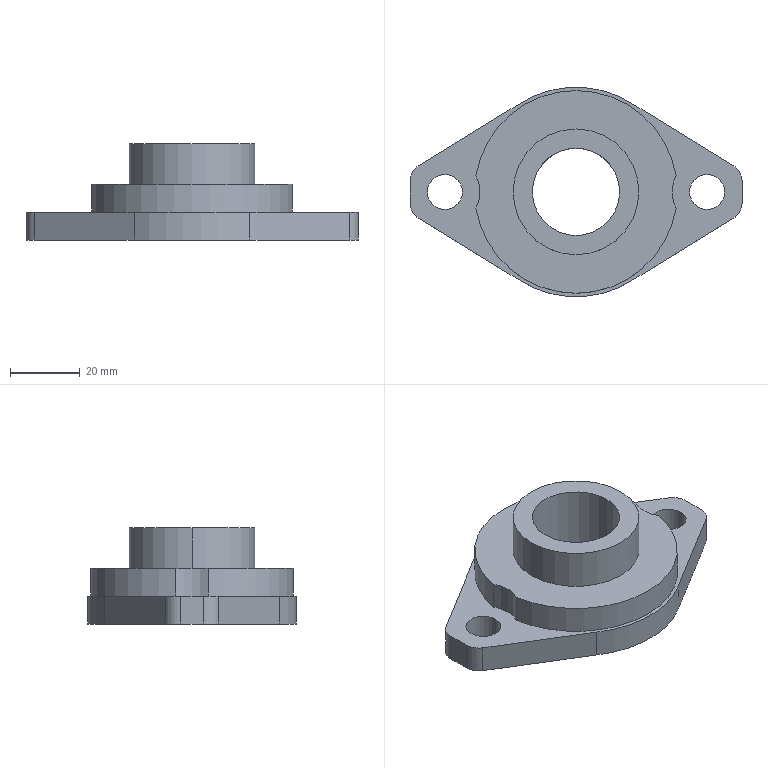Part | SolidWorks | features BaseBody 1 | 1 solid | 32 faces | box 95 x 60 x 27.5 mm | volume 44530 mm3 | cylinder 21 | plane 11 | commonest cylinder face diameters 10 x8 20 x3 25 x2 36 x2 55 x2 58 x2
STEP:
#1=CARTESIAN_POINT('',(12.5,0.,19.5));
#2=VERTEX_POINT('',#1);
#3=CARTESIAN_POINT('',(-12.5,0.,19.5));
#4=VERTEX_POINT('',#3);
#5=CARTESIAN_POINT('',(0.,0.,19.5));
#6=DIRECTION('',(0.,0.,-1.));
#7=DIRECTION('',(-1.,0.,0.));
#8=AXIS2_PLACEMENT_3D('',#5,#6,#7);
#9=CIRCLE('',#8,12.5);
#10=EDGE_CURVE('',#2,#4,#9,.T.);
#11=ORIENTED_EDGE('',*,*,#10,.F.);
#12=CARTESIAN_POINT('',(12.5,0.,-6.));
#13=VERTEX_POINT('',#12);
#14=CARTESIAN_POINT('',(12.5,0.,19.5));
#15=DIRECTION('',(0.,0.,-1.));
#16=VECTOR('',#15,1000.);
#17=LINE('',#14,#16);
#18=EDGE_CURVE('',#2,#13,#17,.T.);
#19=ORIENTED_EDGE('',*,*,#18,.T.);
#20=CARTESIAN_POINT('',(-12.5,0.,-6.));
#21=VERTEX_POINT('',#20);
#22=CARTESIAN_POINT('',(0.,0.,-6.));
#23=DIRECTION('',(0.,0.,1.));
#24=DIRECTION('',(-1.,0.,0.));
#25=AXIS2_PLACEMENT_3D('',#22,#23,#24);
#26=CIRCLE('',#25,12.5);
#27=EDGE_CURVE('',#21,#13,#26,.T.);
#28=ORIENTED_EDGE('',*,*,#27,.F.);
#29=CARTESIAN_POINT('',(-12.5,0.,19.5));
#30=DIRECTION('',(0.,0.,-1.));
#31=VECTOR('',#30,1000.);
#32=LINE('',#29,#31);
#33=EDGE_CURVE('',#4,#21,#32,.T.);
#34=ORIENTED_EDGE('',*,*,#33,.F.);
#35=EDGE_LOOP('',(#11,#19,#28,#34));
#36=FACE_OUTER_BOUND('',#35,.T.);
#37=CARTESIAN_POINT('',(0.,0.,19.5));
#38=DIRECTION('',(0.,0.,-1.));
#39=DIRECTION('',(-1.,0.,0.));
#40=AXIS2_PLACEMENT_3D('',#37,#38,#39);
#41=CYLINDRICAL_SURFACE('',#40,12.5);
#42=ADVANCED_FACE('',(#36),#41,.F.);
#43=CARTESIAN_POINT('',(18.,0.,8.));
#44=VERTEX_POINT('',#43);
#45=CARTESIAN_POINT('',(-18.,0.,8.));
#46=VERTEX_POINT('',#45);
#47=CARTESIAN_POINT('',(0.,0.,8.));
#48=DIRECTION('',(0.,0.,1.));
#49=DIRECTION('',(1.,0.,0.));
#50=AXIS2_PLACEMENT_3D('',#47,#48,#49);
#51=CIRCLE('',#50,18.);
#52=EDGE_CURVE('',#44,#46,#51,.T.);
#53=ORIENTED_EDGE('',*,*,#52,.T.);
#54=CARTESIAN_POINT('',(-18.,0.,19.5));
#55=VERTEX_POINT('',#54);
#56=CARTESIAN_POINT('',(-18.,0.,8.));
#57=DIRECTION('',(0.,0.,1.));
#58=VECTOR('',#57,1000.);
#59=LINE('',#56,#58);
#60=EDGE_CURVE('',#46,#55,#59,.T.);
#61=ORIENTED_EDGE('',*,*,#60,.T.);
#62=CARTESIAN_POINT('',(18.,0.,19.5));
#63=VERTEX_POINT('',#62);
#64=CARTESIAN_POINT('',(0.,0.,19.5));
#65=DIRECTION('',(0.,0.,1.));
#66=DIRECTION('',(1.,0.,0.));
#67=AXIS2_PLACEMENT_3D('',#64,#65,#66);
#68=CIRCLE('',#67,18.);
#69=EDGE_CURVE('',#63,#55,#68,.T.);
#70=ORIENTED_EDGE('',*,*,#69,.F.);
#71=CARTESIAN_POINT('',(18.,0.,8.));
#72=DIRECTION('',(0.,0.,1.));
#73=VECTOR('',#72,1000.);
#74=LINE('',#71,#73);
#75=EDGE_CURVE('',#44,#63,#74,.T.);
#76=ORIENTED_EDGE('',*,*,#75,.F.);
#77=EDGE_LOOP('',(#53,#61,#70,#76));
#78=FACE_OUTER_BOUND('',#77,.T.);
#79=CARTESIAN_POINT('',(0.,0.,8.));
#80=DIRECTION('',(0.,0.,1.));
#81=DIRECTION('',(1.,0.,0.));
#82=AXIS2_PLACEMENT_3D('',#79,#80,#81);
#83=CYLINDRICAL_SURFACE('',#82,18.);
#84=ADVANCED_FACE('',(#78),#83,.T.);
#85=CARTESIAN_POINT('',(-27.5,0.,-8.));
#86=VERTEX_POINT('',#85);
#87=CARTESIAN_POINT('',(27.5,0.,-8.));
#88=VERTEX_POINT('',#87);
#89=CARTESIAN_POINT('',(0.,0.,-8.));
#90=DIRECTION('',(0.,0.,1.));
#91=DIRECTION('',(1.,0.,0.));
#92=AXIS2_PLACEMENT_3D('',#89,#90,#91);
#93=CIRCLE('',#92,27.5);
#94=EDGE_CURVE('',#86,#88,#93,.T.);
#95=ORIENTED_EDGE('',*,*,#94,.F.);
#96=CARTESIAN_POINT('',(-27.5,0.,-6.));
#97=VERTEX_POINT('',#96);
#98=CARTESIAN_POINT('',(-27.5,0.,-8.));
#99=DIRECTION('',(0.,0.,1.));
#100=VECTOR('',#99,1000.);
#101=LINE('',#98,#100);
#102=EDGE_CURVE('',#86,#97,#101,.T.);
#103=ORIENTED_EDGE('',*,*,#102,.T.);
#104=CARTESIAN_POINT('',(27.5,0.,-6.));
#105=VERTEX_POINT('',#104);
#106=CARTESIAN_POINT('',(0.,0.,-6.));
#107=DIRECTION('',(0.,0.,1.));
#108=DIRECTION('',(1.,0.,0.));
#109=AXIS2_PLACEMENT_3D('',#106,#107,#108);
#110=CIRCLE('',#109,27.5);
#111=EDGE_CURVE('',#97,#105,#110,.T.);
#112=ORIENTED_EDGE('',*,*,#111,.T.);
#113=CARTESIAN_POINT('',(27.5,0.,-8.));
#114=DIRECTION('',(0.,0.,1.));
#115=VECTOR('',#114,1000.);
#116=LINE('',#113,#115);
#117=EDGE_CURVE('',#88,#105,#116,.T.);
#118=ORIENTED_EDGE('',*,*,#117,.F.);
#119=EDGE_LOOP('',(#95,#103,#112,#118));
#120=FACE_OUTER_BOUND('',#119,.T.);
#121=CARTESIAN_POINT('',(0.,0.,-8.));
#122=DIRECTION('',(0.,0.,1.));
#123=DIRECTION('',(1.,0.,0.));
#124=AXIS2_PLACEMENT_3D('',#121,#122,#123);
#125=CYLINDRICAL_SURFACE('',#124,27.5);
#126=ADVANCED_FACE('',(#120),#125,.F.);
#127=CARTESIAN_POINT('',(27.5,0.,8.));
#128=VERTEX_POINT('',#127);
#129=CARTESIAN_POINT('',(28.63,4.618,8.));
#130=VERTEX_POINT('',#129);
#131=CARTESIAN_POINT('',(37.5,0.,8.));
#132=DIRECTION('',(0.,0.,-1.));
#133=DIRECTION('',(-1.,0.,0.));
#134=AXIS2_PLACEMENT_3D('',#131,#132,#133);
#135=CIRCLE('',#134,10.);
#136=EDGE_CURVE('',#128,#130,#135,.T.);
#137=ORIENTED_EDGE('',*,*,#136,.F.);
#138=CARTESIAN_POINT('',(27.5,0.,0.));
#139=VERTEX_POINT('',#138);
#140=CARTESIAN_POINT('',(27.5,0.,8.));
#141=DIRECTION('',(0.,0.,-1.));
#142=VECTOR('',#141,1000.);
#143=LINE('',#140,#142);
#144=EDGE_CURVE('',#128,#139,#143,.T.);
#145=ORIENTED_EDGE('',*,*,#144,.T.);
#146=CARTESIAN_POINT('',(28.63,4.618,0.));
#147=VERTEX_POINT('',#146);
#148=CARTESIAN_POINT('',(37.5,0.,0.));
#149=DIRECTION('',(0.,0.,1.));
#150=DIRECTION('',(-1.,0.,0.));
#151=AXIS2_PLACEMENT_3D('',#148,#149,#150);
#152=CIRCLE('',#151,10.);
#153=EDGE_CURVE('',#147,#139,#152,.T.);
#154=ORIENTED_EDGE('',*,*,#153,.F.);
#155=CARTESIAN_POINT('',(28.63,4.618,0.));
#156=DIRECTION('',(0.,0.,-1.));
#157=VECTOR('',#156,1000.);
#158=LINE('',#155,#157);
#159=EDGE_CURVE('',#130,#147,#158,.T.);
#160=ORIENTED_EDGE('',*,*,#159,.F.);
#161=EDGE_LOOP('',(#137,#145,#154,#160));
#162=FACE_OUTER_BOUND('',#161,.T.);
#163=CARTESIAN_POINT('',(37.5,0.,8.));
#164=DIRECTION('',(0.,0.,-1.));
#165=DIRECTION('',(-1.,0.,0.));
#166=AXIS2_PLACEMENT_3D('',#163,#164,#165);
#167=CYLINDRICAL_SURFACE('',#166,10.);
#168=ADVANCED_FACE('',(#162),#167,.F.);
#169=CARTESIAN_POINT('',(32.5,0.,-8.));
#170=VERTEX_POINT('',#169);
#171=CARTESIAN_POINT('',(42.5,0.,-8.));
#172=VERTEX_POINT('',#171);
#173=CARTESIAN_POINT('',(37.5,0.,-8.));
#174=DIRECTION('',(0.,0.,1.));
#175=DIRECTION('',(1.,0.,0.));
#176=AXIS2_PLACEMENT_3D('',#173,#174,#175);
#177=CIRCLE('',#176,5.);
#178=EDGE_CURVE('',#170,#172,#177,.T.);
#179=ORIENTED_EDGE('',*,*,#178,.F.);
#180=CARTESIAN_POINT('',(32.5,0.,0.));
#181=VERTEX_POINT('',#180);
#182=CARTESIAN_POINT('',(32.5,0.,-8.));
#183=DIRECTION('',(0.,0.,1.));
#184=VECTOR('',#183,1000.);
#185=LINE('',#182,#184);
#186=EDGE_CURVE('',#170,#181,#185,.T.);
#187=ORIENTED_EDGE('',*,*,#186,.T.);
#188=CARTESIAN_POINT('',(42.5,0.,0.));
#189=VERTEX_POINT('',#188);
#190=CARTESIAN_POINT('',(37.5,0.,0.));
#191=DIRECTION('',(0.,0.,-1.));
#192=DIRECTION('',(1.,0.,0.));
#193=AXIS2_PLACEMENT_3D('',#190,#191,#192);
#194=CIRCLE('',#193,5.);
#195=EDGE_CURVE('',#189,#181,#194,.T.);
#196=ORIENTED_EDGE('',*,*,#195,.F.);
#197=CARTESIAN_POINT('',(42.5,0.,-8.));
#198=DIRECTION('',(0.,0.,1.));
#199=VECTOR('',#198,1000.);
#200=LINE('',#197,#199);
#201=EDGE_CURVE('',#172,#189,#200,.T.);
#202=ORIENTED_EDGE('',*,*,#201,.F.);
#203=EDGE_LOOP('',(#179,#187,#196,#202));
#204=FACE_OUTER_BOUND('',#203,.T.);
#205=CARTESIAN_POINT('',(37.5,0.,-8.));
#206=DIRECTION('',(0.,0.,1.));
#207=DIRECTION('',(1.,0.,0.));
#208=AXIS2_PLACEMENT_3D('',#205,#206,#207);
#209=CYLINDRICAL_SURFACE('',#208,5.);
#210=ADVANCED_FACE('',(#204),#209,.F.);
#211=CARTESIAN_POINT('',(-42.5,0.,-8.));
#212=VERTEX_POINT('',#211);
#213=CARTESIAN_POINT('',(-32.5,0.,-8.));
#214=VERTEX_POINT('',#213);
#215=CARTESIAN_POINT('',(-37.5,0.,-8.));
#216=DIRECTION('',(0.,0.,1.));
#217=DIRECTION('',(1.,0.,0.));
#218=AXIS2_PLACEMENT_3D('',#215,#216,#217);
#219=CIRCLE('',#218,5.);
#220=EDGE_CURVE('',#212,#214,#219,.T.);
#221=ORIENTED_EDGE('',*,*,#220,.F.);
#222=CARTESIAN_POINT('',(-42.5,0.,0.));
#223=VERTEX_POINT('',#222);
#224=CARTESIAN_POINT('',(-42.5,0.,-8.));
#225=DIRECTION('',(0.,0.,1.));
#226=VECTOR('',#225,1000.);
#227=LINE('',#224,#226);
#228=EDGE_CURVE('',#212,#223,#227,.T.);
#229=ORIENTED_EDGE('',*,*,#228,.T.);
#230=CARTESIAN_POINT('',(-32.5,0.,0.));
#231=VERTEX_POINT('',#230);
#232=CARTESIAN_POINT('',(-37.5,0.,0.));
#233=DIRECTION('',(0.,0.,-1.));
#234=DIRECTION('',(1.,0.,0.));
#235=AXIS2_PLACEMENT_3D('',#232,#233,#234);
#236=CIRCLE('',#235,5.);
#237=EDGE_CURVE('',#231,#223,#236,.T.);
#238=ORIENTED_EDGE('',*,*,#237,.F.);
#239=CARTESIAN_POINT('',(-32.5,0.,-8.));
#240=DIRECTION('',(0.,0.,1.));
#241=VECTOR('',#240,1000.);
#242=LINE('',#239,#241);
#243=EDGE_CURVE('',#214,#231,#242,.T.);
#244=ORIENTED_EDGE('',*,*,#243,.F.);
#245=EDGE_LOOP('',(#221,#229,#238,#244));
#246=FACE_OUTER_BOUND('',#245,.T.);
#247=CARTESIAN_POINT('',(-37.5,0.,-8.));
#248=DIRECTION('',(0.,0.,1.));
#249=DIRECTION('',(1.,0.,0.));
#250=AXIS2_PLACEMENT_3D('',#247,#248,#249);
#251=CYLINDRICAL_SURFACE('',#250,5.);
#252=ADVANCED_FACE('',(#246),#251,.F.);
#253=ORIENTED_EDGE('',*,*,#18,.F.);
#254=CARTESIAN_POINT('',(0.,0.,19.5));
#255=DIRECTION('',(0.,0.,-1.));
#256=DIRECTION('',(-1.,0.,0.));
#257=AXIS2_PLACEMENT_3D('',#254,#255,#256);
#258=CIRCLE('',#257,12.5);
#259=EDGE_CURVE('',#4,#2,#258,.T.);
#260=ORIENTED_EDGE('',*,*,#259,.F.);
#261=ORIENTED_EDGE('',*,*,#33,.T.);
#262=CARTESIAN_POINT('',(0.,0.,-6.));
#263=DIRECTION('',(0.,0.,1.));
#264=DIRECTION('',(-1.,0.,0.));
#265=AXIS2_PLACEMENT_3D('',#262,#263,#264);
#266=CIRCLE('',#265,12.5);
#267=EDGE_CURVE('',#13,#21,#266,.T.);
#268=ORIENTED_EDGE('',*,*,#267,.F.);
#269=EDGE_LOOP('',(#253,#260,#261,#268));
#270=FACE_OUTER_BOUND('',#269,.T.);
#271=CARTESIAN_POINT('',(0.,0.,19.5));
#272=DIRECTION('',(0.,0.,-1.));
#273=DIRECTION('',(-1.,0.,0.));
#274=AXIS2_PLACEMENT_3D('',#271,#272,#273);
#275=CYLINDRICAL_SURFACE('',#274,12.5);
#276=ADVANCED_FACE('',(#270),#275,.F.);
#277=ORIENTED_EDGE('',*,*,#69,.T.);
#278=CARTESIAN_POINT('',(0.,0.,19.5));
#279=DIRECTION('',(0.,0.,1.));
#280=DIRECTION('',(1.,0.,0.));
#281=AXIS2_PLACEMENT_3D('',#278,#279,#280);
#282=CIRCLE('',#281,18.);
#283=EDGE_CURVE('',#55,#63,#282,.T.);
#284=ORIENTED_EDGE('',*,*,#283,.T.);
#285=EDGE_LOOP('',(#277,#284));
#286=FACE_OUTER_BOUND('',#285,.T.);
#287=ORIENTED_EDGE('',*,*,#259,.T.);
#288=ORIENTED_EDGE('',*,*,#10,.T.);
#289=EDGE_LOOP('',(#287,#288));
#290=FACE_BOUND('',#289,.T.);
#291=CARTESIAN_POINT('',(0.,0.,19.5));
#292=DIRECTION('',(0.,0.,1.));
#293=DIRECTION('',(1.,0.,0.));
#294=AXIS2_PLACEMENT_3D('',#291,#292,#293);
#295=PLANE('',#294);
#296=ADVANCED_FACE('',(#286,#290),#295,.T.);
#297=ORIENTED_EDGE('',*,*,#27,.T.);
#298=ORIENTED_EDGE('',*,*,#267,.T.);
#299=EDGE_LOOP('',(#297,#298));
#300=FACE_BOUND('',#299,.T.);
#301=CARTESIAN_POINT('',(0.,0.,-6.));
#302=DIRECTION('',(0.,0.,1.));
#303=DIRECTION('',(1.,0.,0.));
#304=AXIS2_PLACEMENT_3D('',#301,#302,#303);
#305=CIRCLE('',#304,27.5);
#306=EDGE_CURVE('',#105,#97,#305,.T.);
#307=ORIENTED_EDGE('',*,*,#306,.F.);
#308=ORIENTED_EDGE('',*,*,#111,.F.);
#309=EDGE_LOOP('',(#307,#308));
#310=FACE_OUTER_BOUND('',#309,.T.);
#311=CARTESIAN_POINT('',(0.,0.,-6.));
#312=DIRECTION('',(0.,0.,1.));
#313=DIRECTION('',(1.,0.,0.));
#314=AXIS2_PLACEMENT_3D('',#311,#312,#313);
#315=PLANE('',#314);
#316=ADVANCED_FACE('',(#300,#310),#315,.F.);
#317=ORIENTED_EDGE('',*,*,#60,.F.);
#318=CARTESIAN_POINT('',(0.,0.,8.));
#319=DIRECTION('',(0.,0.,1.));
#320=DIRECTION('',(1.,0.,0.));
#321=AXIS2_PLACEMENT_3D('',#318,#319,#320);
#322=CIRCLE('',#321,18.);
#323=EDGE_CURVE('',#46,#44,#322,.T.);
#324=ORIENTED_EDGE('',*,*,#323,.T.);
#325=ORIENTED_EDGE('',*,*,#75,.T.);
#326=ORIENTED_EDGE('',*,*,#283,.F.);
#327=EDGE_LOOP('',(#317,#324,#325,#326));
#328=FACE_OUTER_BOUND('',#327,.T.);
#329=CARTESIAN_POINT('',(0.,0.,8.));
#330=DIRECTION('',(0.,0.,1.));
#331=DIRECTION('',(1.,0.,0.));
#332=AXIS2_PLACEMENT_3D('',#329,#330,#331);
#333=CYLINDRICAL_SURFACE('',#332,18.);
#334=ADVANCED_FACE('',(#328),#333,.T.);
#335=ORIENTED_EDGE('',*,*,#102,.F.);
#336=CARTESIAN_POINT('',(0.,0.,-8.));
#337=DIRECTION('',(0.,0.,1.));
#338=DIRECTION('',(1.,0.,0.));
#339=AXIS2_PLACEMENT_3D('',#336,#337,#338);
#340=CIRCLE('',#339,27.5);
#341=EDGE_CURVE('',#88,#86,#340,.T.);
#342=ORIENTED_EDGE('',*,*,#341,.F.);
#343=ORIENTED_EDGE('',*,*,#117,.T.);
#344=ORIENTED_EDGE('',*,*,#306,.T.);
#345=EDGE_LOOP('',(#335,#342,#343,#344));
#346=FACE_OUTER_BOUND('',#345,.T.);
#347=CARTESIAN_POINT('',(0.,0.,-8.));
#348=DIRECTION('',(0.,0.,1.));
#349=DIRECTION('',(1.,0.,0.));
#350=AXIS2_PLACEMENT_3D('',#347,#348,#349);
#351=CYLINDRICAL_SURFACE('',#350,27.5);
#352=ADVANCED_FACE('',(#346),#351,.F.);
#353=ORIENTED_EDGE('',*,*,#52,.F.);
#354=ORIENTED_EDGE('',*,*,#323,.F.);
#355=EDGE_LOOP('',(#353,#354));
#356=FACE_BOUND('',#355,.T.);
#357=CARTESIAN_POINT('',(-28.63,4.618,8.));
#358=VERTEX_POINT('',#357);
#359=CARTESIAN_POINT('',(-28.63,-4.618,8.));
#360=VERTEX_POINT('',#359);
#361=CARTESIAN_POINT('',(-37.5,0.,8.));
#362=DIRECTION('',(0.,0.,-1.));
#363=DIRECTION('',(-1.,0.,0.));
#364=AXIS2_PLACEMENT_3D('',#361,#362,#363);
#365=CIRCLE('',#364,10.);
#366=EDGE_CURVE('',#358,#360,#365,.T.);
#367=ORIENTED_EDGE('',*,*,#366,.T.);
#368=CARTESIAN_POINT('',(28.63,-4.618,8.));
#369=VERTEX_POINT('',#368);
#370=CARTESIAN_POINT('',(0.,0.,8.));
#371=DIRECTION('',(0.,0.,1.));
#372=DIRECTION('',(1.,0.,0.));
#373=AXIS2_PLACEMENT_3D('',#370,#371,#372);
#374=CIRCLE('',#373,29.);
#375=EDGE_CURVE('',#360,#369,#374,.T.);
#376=ORIENTED_EDGE('',*,*,#375,.T.);
#377=CARTESIAN_POINT('',(37.5,0.,8.));
#378=DIRECTION('',(0.,0.,-1.));
#379=DIRECTION('',(-1.,0.,0.));
#380=AXIS2_PLACEMENT_3D('',#377,#378,#379);
#381=CIRCLE('',#380,10.);
#382=EDGE_CURVE('',#369,#128,#381,.T.);
#383=ORIENTED_EDGE('',*,*,#382,.T.);
#384=ORIENTED_EDGE('',*,*,#136,.T.);
#385=CARTESIAN_POINT('',(0.,0.,8.));
#386=DIRECTION('',(0.,0.,1.));
#387=DIRECTION('',(1.,0.,0.));
#388=AXIS2_PLACEMENT_3D('',#385,#386,#387);
#389=CIRCLE('',#388,29.);
#390=EDGE_CURVE('',#130,#358,#389,.T.);
#391=ORIENTED_EDGE('',*,*,#390,.T.);
#392=EDGE_LOOP('',(#367,#376,#383,#384,#391));
#393=FACE_OUTER_BOUND('',#392,.T.);
#394=CARTESIAN_POINT('',(0.,0.,8.));
#395=DIRECTION('',(0.,0.,1.));
#396=DIRECTION('',(1.,0.,0.));
#397=AXIS2_PLACEMENT_3D('',#394,#395,#396);
#398=PLANE('',#397);
#399=ADVANCED_FACE('',(#356,#393),#398,.T.);
#400=CARTESIAN_POINT('',(37.5,0.,-8.));
#401=DIRECTION('',(0.,0.,1.));
#402=DIRECTION('',(1.,0.,0.));
#403=AXIS2_PLACEMENT_3D('',#400,#401,#402);
#404=CIRCLE('',#403,5.);
#405=EDGE_CURVE('',#172,#170,#404,.T.);
#406=ORIENTED_EDGE('',*,*,#405,.T.);
#407=ORIENTED_EDGE('',*,*,#178,.T.);
#408=EDGE_LOOP('',(#406,#407));
#409=FACE_BOUND('',#408,.T.);
#410=CARTESIAN_POINT('',(-37.5,0.,-8.));
#411=DIRECTION('',(0.,0.,1.));
#412=DIRECTION('',(1.,0.,0.));
#413=AXIS2_PLACEMENT_3D('',#410,#411,#412);
#414=CIRCLE('',#413,5.);
#415=EDGE_CURVE('',#214,#212,#414,.T.);
#416=ORIENTED_EDGE('',*,*,#415,.T.);
#417=ORIENTED_EDGE('',*,*,#220,.T.);
#418=EDGE_LOOP('',(#416,#417));
#419=FACE_BOUND('',#418,.T.);
#420=CARTESIAN_POINT('',(16.583,25.,-8.));
#421=VERTEX_POINT('',#420);
#422=CARTESIAN_POINT('',(45.118,7.464,-8.));
#423=VERTEX_POINT('',#422);
#424=CARTESIAN_POINT('',(16.583,25.,-8.));
#425=DIRECTION('',(0.852,-0.5236,0.));
#426=VECTOR('',#425,1000.);
#427=LINE('',#424,#426);
#428=EDGE_CURVE('',#421,#423,#427,.T.);
#429=ORIENTED_EDGE('',*,*,#428,.T.);
#430=CARTESIAN_POINT('',(47.5,3.204,-8.));
#431=VERTEX_POINT('',#430);
#432=CARTESIAN_POINT('',(42.5,3.204,-8.));
#433=DIRECTION('',(0.,0.,-1.));
#434=DIRECTION('',(1.,0.,0.));
#435=AXIS2_PLACEMENT_3D('',#432,#433,#434);
#436=CIRCLE('',#435,5.);
#437=EDGE_CURVE('',#423,#431,#436,.T.);
#438=ORIENTED_EDGE('',*,*,#437,.T.);
#439=CARTESIAN_POINT('',(47.5,-3.204,-8.));
#440=VERTEX_POINT('',#439);
#441=CARTESIAN_POINT('',(47.5,0.,-8.));
#442=DIRECTION('',(0.,-1.,0.));
#443=VECTOR('',#442,1000.);
#444=LINE('',#441,#443);
#445=EDGE_CURVE('',#431,#440,#444,.T.);
#446=ORIENTED_EDGE('',*,*,#445,.T.);
#447=CARTESIAN_POINT('',(45.118,-7.464,-8.));
#448=VERTEX_POINT('',#447);
#449=CARTESIAN_POINT('',(42.5,-3.204,-8.));
#450=DIRECTION('',(0.,0.,-1.));
#451=DIRECTION('',(1.,0.,0.));
#452=AXIS2_PLACEMENT_3D('',#449,#450,#451);
#453=CIRCLE('',#452,5.);
#454=EDGE_CURVE('',#440,#448,#453,.T.);
#455=ORIENTED_EDGE('',*,*,#454,.T.);
#456=CARTESIAN_POINT('',(16.583,-25.,-8.));
#457=VERTEX_POINT('',#456);
#458=CARTESIAN_POINT('',(45.118,-7.464,-8.));
#459=DIRECTION('',(-0.852,-0.5236,0.));
#460=VECTOR('',#459,1000.);
#461=LINE('',#458,#460);
#462=EDGE_CURVE('',#448,#457,#461,.T.);
#463=ORIENTED_EDGE('',*,*,#462,.T.);
#464=CARTESIAN_POINT('',(-16.583,-25.,-8.));
#465=VERTEX_POINT('',#464);
#466=CARTESIAN_POINT('',(0.,0.,-8.));
#467=DIRECTION('',(0.,0.,-1.));
#468=DIRECTION('',(1.,0.,0.));
#469=AXIS2_PLACEMENT_3D('',#466,#467,#468);
#470=CIRCLE('',#469,30.);
#471=EDGE_CURVE('',#457,#465,#470,.T.);
#472=ORIENTED_EDGE('',*,*,#471,.T.);
#473=CARTESIAN_POINT('',(-45.118,-7.464,-8.));
#474=VERTEX_POINT('',#473);
#475=CARTESIAN_POINT('',(-16.583,-25.,-8.));
#476=DIRECTION('',(-0.852,0.5236,0.));
#477=VECTOR('',#476,1000.);
#478=LINE('',#475,#477);
#479=EDGE_CURVE('',#465,#474,#478,.T.);
#480=ORIENTED_EDGE('',*,*,#479,.T.);
#481=CARTESIAN_POINT('',(-47.5,-3.204,-8.));
#482=VERTEX_POINT('',#481);
#483=CARTESIAN_POINT('',(-42.5,-3.204,-8.));
#484=DIRECTION('',(0.,0.,-1.));
#485=DIRECTION('',(1.,0.,0.));
#486=AXIS2_PLACEMENT_3D('',#483,#484,#485);
#487=CIRCLE('',#486,5.);
#488=EDGE_CURVE('',#474,#482,#487,.T.);
#489=ORIENTED_EDGE('',*,*,#488,.T.);
#490=CARTESIAN_POINT('',(-47.5,3.204,-8.));
#491=VERTEX_POINT('',#490);
#492=CARTESIAN_POINT('',(-47.5,0.,-8.));
#493=DIRECTION('',(0.,1.,0.));
#494=VECTOR('',#493,1000.);
#495=LINE('',#492,#494);
#496=EDGE_CURVE('',#482,#491,#495,.T.);
#497=ORIENTED_EDGE('',*,*,#496,.T.);
#498=CARTESIAN_POINT('',(-45.118,7.464,-8.));
#499=VERTEX_POINT('',#498);
#500=CARTESIAN_POINT('',(-42.5,3.204,-8.));
#501=DIRECTION('',(0.,0.,-1.));
#502=DIRECTION('',(1.,0.,0.));
#503=AXIS2_PLACEMENT_3D('',#500,#501,#502);
#504=CIRCLE('',#503,5.);
#505=EDGE_CURVE('',#491,#499,#504,.T.);
#506=ORIENTED_EDGE('',*,*,#505,.T.);
#507=CARTESIAN_POINT('',(-16.583,25.,-8.));
#508=VERTEX_POINT('',#507);
#509=CARTESIAN_POINT('',(-45.118,7.464,-8.));
#510=DIRECTION('',(0.852,0.5236,0.));
#511=VECTOR('',#510,1000.);
#512=LINE('',#509,#511);
#513=EDGE_CURVE('',#499,#508,#512,.T.);
#514=ORIENTED_EDGE('',*,*,#513,.T.);
#515=CARTESIAN_POINT('',(0.,0.,-8.));
#516=DIRECTION('',(0.,0.,-1.));
#517=DIRECTION('',(1.,0.,0.));
#518=AXIS2_PLACEMENT_3D('',#515,#516,#517);
#519=CIRCLE('',#518,30.);
#520=EDGE_CURVE('',#508,#421,#519,.T.);
#521=ORIENTED_EDGE('',*,*,#520,.T.);
#522=EDGE_LOOP('',(#429,#438,#446,#455,#463,#472,#480,#489,#497,#506,#514,#521));
#523=FACE_OUTER_BOUND('',#522,.T.);
#524=ORIENTED_EDGE('',*,*,#341,.T.);
#525=ORIENTED_EDGE('',*,*,#94,.T.);
#526=EDGE_LOOP('',(#524,#525));
#527=FACE_BOUND('',#526,.T.);
#528=CARTESIAN_POINT('',(0.,0.,-8.));
#529=DIRECTION('',(0.,0.,-1.));
#530=DIRECTION('',(-1.,0.,0.));
#531=AXIS2_PLACEMENT_3D('',#528,#529,#530);
#532=PLANE('',#531);
#533=ADVANCED_FACE('',(#409,#419,#523,#527),#532,.T.);
#534=CARTESIAN_POINT('',(-28.63,-4.618,0.));
#535=VERTEX_POINT('',#534);
#536=CARTESIAN_POINT('',(-28.63,-4.618,0.));
#537=DIRECTION('',(0.,0.,-1.));
#538=VECTOR('',#537,1000.);
#539=LINE('',#536,#538);
#540=EDGE_CURVE('',#360,#535,#539,.T.);
#541=ORIENTED_EDGE('',*,*,#540,.T.);
#542=CARTESIAN_POINT('',(28.63,-4.618,0.));
#543=VERTEX_POINT('',#542);
#544=CARTESIAN_POINT('',(0.,0.,0.));
#545=DIRECTION('',(0.,0.,1.));
#546=DIRECTION('',(1.,0.,0.));
#547=AXIS2_PLACEMENT_3D('',#544,#545,#546);
#548=CIRCLE('',#547,29.);
#549=EDGE_CURVE('',#535,#543,#548,.T.);
#550=ORIENTED_EDGE('',*,*,#549,.T.);
#551=CARTESIAN_POINT('',(28.63,-4.618,0.));
#552=DIRECTION('',(0.,0.,1.));
#553=VECTOR('',#552,1000.);
#554=LINE('',#551,#553);
#555=EDGE_CURVE('',#543,#369,#554,.T.);
#556=ORIENTED_EDGE('',*,*,#555,.T.);
#557=ORIENTED_EDGE('',*,*,#375,.F.);
#558=EDGE_LOOP('',(#541,#550,#556,#557));
#559=FACE_OUTER_BOUND('',#558,.T.);
#560=CARTESIAN_POINT('',(0.,0.,0.));
#561=DIRECTION('',(0.,0.,1.));
#562=DIRECTION('',(1.,0.,0.));
#563=AXIS2_PLACEMENT_3D('',#560,#561,#562);
#564=CYLINDRICAL_SURFACE('',#563,29.);
#565=ADVANCED_FACE('',(#559),#564,.T.);
#566=ORIENTED_EDGE('',*,*,#366,.F.);
#567=CARTESIAN_POINT('',(-28.63,4.618,0.));
#568=VERTEX_POINT('',#567);
#569=CARTESIAN_POINT('',(-28.63,4.618,8.));
#570=DIRECTION('',(0.,0.,1.));
#571=VECTOR('',#570,1000.);
#572=LINE('',#569,#571);
#573=EDGE_CURVE('',#568,#358,#572,.T.);
#574=ORIENTED_EDGE('',*,*,#573,.F.);
#575=CARTESIAN_POINT('',(-37.5,0.,0.));
#576=DIRECTION('',(0.,0.,1.));
#577=DIRECTION('',(-1.,0.,0.));
#578=AXIS2_PLACEMENT_3D('',#575,#576,#577);
#579=CIRCLE('',#578,10.);
#580=EDGE_CURVE('',#535,#568,#579,.T.);
#581=ORIENTED_EDGE('',*,*,#580,.F.);
#582=ORIENTED_EDGE('',*,*,#540,.F.);
#583=EDGE_LOOP('',(#566,#574,#581,#582));
#584=FACE_OUTER_BOUND('',#583,.T.);
#585=CARTESIAN_POINT('',(-37.5,0.,8.));
#586=DIRECTION('',(0.,0.,-1.));
#587=DIRECTION('',(-1.,0.,0.));
#588=AXIS2_PLACEMENT_3D('',#585,#586,#587);
#589=CYLINDRICAL_SURFACE('',#588,10.);
#590=ADVANCED_FACE('',(#584),#589,.F.);
#591=ORIENTED_EDGE('',*,*,#573,.T.);
#592=ORIENTED_EDGE('',*,*,#390,.F.);
#593=ORIENTED_EDGE('',*,*,#159,.T.);
#594=CARTESIAN_POINT('',(0.,0.,0.));
#595=DIRECTION('',(0.,0.,1.));
#596=DIRECTION('',(1.,0.,0.));
#597=AXIS2_PLACEMENT_3D('',#594,#595,#596);
#598=CIRCLE('',#597,29.);
#599=EDGE_CURVE('',#147,#568,#598,.T.);
#600=ORIENTED_EDGE('',*,*,#599,.T.);
#601=EDGE_LOOP('',(#591,#592,#593,#600));
#602=FACE_OUTER_BOUND('',#601,.T.);
#603=CARTESIAN_POINT('',(0.,0.,0.));
#604=DIRECTION('',(0.,0.,1.));
#605=DIRECTION('',(1.,0.,0.));
#606=AXIS2_PLACEMENT_3D('',#603,#604,#605);
#607=CYLINDRICAL_SURFACE('',#606,29.);
#608=ADVANCED_FACE('',(#602),#607,.T.);
#609=ORIENTED_EDGE('',*,*,#144,.F.);
#610=ORIENTED_EDGE('',*,*,#382,.F.);
#611=ORIENTED_EDGE('',*,*,#555,.F.);
#612=CARTESIAN_POINT('',(37.5,0.,0.));
#613=DIRECTION('',(0.,0.,1.));
#614=DIRECTION('',(-1.,0.,0.));
#615=AXIS2_PLACEMENT_3D('',#612,#613,#614);
#616=CIRCLE('',#615,10.);
#617=EDGE_CURVE('',#139,#543,#616,.T.);
#618=ORIENTED_EDGE('',*,*,#617,.F.);
#619=EDGE_LOOP('',(#609,#610,#611,#618));
#620=FACE_OUTER_BOUND('',#619,.T.);
#621=CARTESIAN_POINT('',(37.5,0.,8.));
#622=DIRECTION('',(0.,0.,-1.));
#623=DIRECTION('',(-1.,0.,0.));
#624=AXIS2_PLACEMENT_3D('',#621,#622,#623);
#625=CYLINDRICAL_SURFACE('',#624,10.);
#626=ADVANCED_FACE('',(#620),#625,.F.);
#627=ORIENTED_EDGE('',*,*,#186,.F.);
#628=ORIENTED_EDGE('',*,*,#405,.F.);
#629=ORIENTED_EDGE('',*,*,#201,.T.);
#630=CARTESIAN_POINT('',(37.5,0.,0.));
#631=DIRECTION('',(0.,0.,-1.));
#632=DIRECTION('',(1.,0.,0.));
#633=AXIS2_PLACEMENT_3D('',#630,#631,#632);
#634=CIRCLE('',#633,5.);
#635=EDGE_CURVE('',#181,#189,#634,.T.);
#636=ORIENTED_EDGE('',*,*,#635,.F.);
#637=EDGE_LOOP('',(#627,#628,#629,#636));
#638=FACE_OUTER_BOUND('',#637,.T.);
#639=CARTESIAN_POINT('',(37.5,0.,-8.));
#640=DIRECTION('',(0.,0.,1.));
#641=DIRECTION('',(1.,0.,0.));
#642=AXIS2_PLACEMENT_3D('',#639,#640,#641);
#643=CYLINDRICAL_SURFACE('',#642,5.);
#644=ADVANCED_FACE('',(#638),#643,.F.);
#645=ORIENTED_EDGE('',*,*,#228,.F.);
#646=ORIENTED_EDGE('',*,*,#415,.F.);
#647=ORIENTED_EDGE('',*,*,#243,.T.);
#648=CARTESIAN_POINT('',(-37.5,0.,0.));
#649=DIRECTION('',(0.,0.,-1.));
#650=DIRECTION('',(1.,0.,0.));
#651=AXIS2_PLACEMENT_3D('',#648,#649,#650);
#652=CIRCLE('',#651,5.);
#653=EDGE_CURVE('',#223,#231,#652,.T.);
#654=ORIENTED_EDGE('',*,*,#653,.F.);
#655=EDGE_LOOP('',(#645,#646,#647,#654));
#656=FACE_OUTER_BOUND('',#655,.T.);
#657=CARTESIAN_POINT('',(-37.5,0.,-8.));
#658=DIRECTION('',(0.,0.,1.));
#659=DIRECTION('',(1.,0.,0.));
#660=AXIS2_PLACEMENT_3D('',#657,#658,#659);
#661=CYLINDRICAL_SURFACE('',#660,5.);
#662=ADVANCED_FACE('',(#656),#661,.F.);
#663=CARTESIAN_POINT('',(45.118,7.464,0.));
#664=VERTEX_POINT('',#663);
#665=CARTESIAN_POINT('',(47.5,3.204,0.));
#666=VERTEX_POINT('',#665);
#667=CARTESIAN_POINT('',(42.5,3.204,0.));
#668=DIRECTION('',(0.,0.,-1.));
#669=DIRECTION('',(1.,0.,0.));
#670=AXIS2_PLACEMENT_3D('',#667,#668,#669);
#671=CIRCLE('',#670,5.);
#672=EDGE_CURVE('',#664,#666,#671,.T.);
#673=ORIENTED_EDGE('',*,*,#672,.T.);
#674=CARTESIAN_POINT('',(47.5,3.204,-8.));
#675=DIRECTION('',(0.,0.,-1.));
#676=VECTOR('',#675,1000.);
#677=LINE('',#674,#676);
#678=EDGE_CURVE('',#666,#431,#677,.T.);
#679=ORIENTED_EDGE('',*,*,#678,.T.);
#680=ORIENTED_EDGE('',*,*,#437,.F.);
#681=CARTESIAN_POINT('',(45.118,7.464,-8.));
#682=DIRECTION('',(0.,0.,1.));
#683=VECTOR('',#682,1000.);
#684=LINE('',#681,#683);
#685=EDGE_CURVE('',#423,#664,#684,.T.);
#686=ORIENTED_EDGE('',*,*,#685,.T.);
#687=EDGE_LOOP('',(#673,#679,#680,#686));
#688=FACE_OUTER_BOUND('',#687,.T.);
#689=CARTESIAN_POINT('',(42.5,3.204,-8.));
#690=DIRECTION('',(0.,0.,1.));
#691=DIRECTION('',(1.,0.,0.));
#692=AXIS2_PLACEMENT_3D('',#689,#690,#691);
#693=CYLINDRICAL_SURFACE('',#692,5.);
#694=ADVANCED_FACE('',(#688),#693,.T.);
#695=ORIENTED_EDGE('',*,*,#685,.F.);
#696=ORIENTED_EDGE('',*,*,#428,.F.);
#697=CARTESIAN_POINT('',(16.583,25.,0.));
#698=VERTEX_POINT('',#697);
#699=CARTESIAN_POINT('',(16.583,25.,-8.));
#700=DIRECTION('',(0.,0.,-1.));
#701=VECTOR('',#700,1000.);
#702=LINE('',#699,#701);
#703=EDGE_CURVE('',#698,#421,#702,.T.);
#704=ORIENTED_EDGE('',*,*,#703,.F.);
#705=CARTESIAN_POINT('',(16.583,25.,0.));
#706=DIRECTION('',(-0.852,0.5236,0.));
#707=VECTOR('',#706,1000.);
#708=LINE('',#705,#707);
#709=EDGE_CURVE('',#664,#698,#708,.T.);
#710=ORIENTED_EDGE('',*,*,#709,.F.);
#711=EDGE_LOOP('',(#695,#696,#704,#710));
#712=FACE_OUTER_BOUND('',#711,.T.);
#713=CARTESIAN_POINT('',(16.583,25.,-8.));
#714=DIRECTION('',(-0.5236,-0.852,0.));
#715=DIRECTION('',(0.852,-0.5236,0.));
#716=AXIS2_PLACEMENT_3D('',#713,#714,#715);
#717=PLANE('',#716);
#718=ADVANCED_FACE('',(#712),#717,.F.);
#719=ORIENTED_EDGE('',*,*,#520,.F.);
#720=CARTESIAN_POINT('',(-16.583,25.,0.));
#721=VERTEX_POINT('',#720);
#722=CARTESIAN_POINT('',(-16.583,25.,-8.));
#723=DIRECTION('',(0.,0.,1.));
#724=VECTOR('',#723,1000.);
#725=LINE('',#722,#724);
#726=EDGE_CURVE('',#508,#721,#725,.T.);
#727=ORIENTED_EDGE('',*,*,#726,.T.);
#728=CARTESIAN_POINT('',(0.,0.,0.));
#729=DIRECTION('',(0.,0.,-1.));
#730=DIRECTION('',(1.,0.,0.));
#731=AXIS2_PLACEMENT_3D('',#728,#729,#730);
#732=CIRCLE('',#731,30.);
#733=EDGE_CURVE('',#721,#698,#732,.T.);
#734=ORIENTED_EDGE('',*,*,#733,.T.);
#735=ORIENTED_EDGE('',*,*,#703,.T.);
#736=EDGE_LOOP('',(#719,#727,#734,#735));
#737=FACE_OUTER_BOUND('',#736,.T.);
#738=CARTESIAN_POINT('',(0.,0.,-8.));
#739=DIRECTION('',(0.,0.,1.));
#740=DIRECTION('',(1.,0.,0.));
#741=AXIS2_PLACEMENT_3D('',#738,#739,#740);
#742=CYLINDRICAL_SURFACE('',#741,30.);
#743=ADVANCED_FACE('',(#737),#742,.T.);
#744=CARTESIAN_POINT('',(-45.118,7.464,0.));
#745=VERTEX_POINT('',#744);
#746=CARTESIAN_POINT('',(-45.118,7.464,-8.));
#747=DIRECTION('',(0.,0.,-1.));
#748=VECTOR('',#747,1000.);
#749=LINE('',#746,#748);
#750=EDGE_CURVE('',#745,#499,#749,.T.);
#751=ORIENTED_EDGE('',*,*,#750,.F.);
#752=CARTESIAN_POINT('',(-47.5,6.,0.));
#753=DIRECTION('',(-0.852,-0.5236,0.));
#754=VECTOR('',#753,1000.);
#755=LINE('',#752,#754);
#756=EDGE_CURVE('',#721,#745,#755,.T.);
#757=ORIENTED_EDGE('',*,*,#756,.F.);
#758=ORIENTED_EDGE('',*,*,#726,.F.);
#759=ORIENTED_EDGE('',*,*,#513,.F.);
#760=EDGE_LOOP('',(#751,#757,#758,#759));
#761=FACE_OUTER_BOUND('',#760,.T.);
#762=CARTESIAN_POINT('',(-47.5,6.,-8.));
#763=DIRECTION('',(0.5236,-0.852,0.));
#764=DIRECTION('',(0.852,0.5236,0.));
#765=AXIS2_PLACEMENT_3D('',#762,#763,#764);
#766=PLANE('',#765);
#767=ADVANCED_FACE('',(#761),#766,.F.);
#768=CARTESIAN_POINT('',(-47.5,3.204,0.));
#769=VERTEX_POINT('',#768);
#770=CARTESIAN_POINT('',(-42.5,3.204,0.));
#771=DIRECTION('',(0.,0.,-1.));
#772=DIRECTION('',(1.,0.,0.));
#773=AXIS2_PLACEMENT_3D('',#770,#771,#772);
#774=CIRCLE('',#773,5.);
#775=EDGE_CURVE('',#769,#745,#774,.T.);
#776=ORIENTED_EDGE('',*,*,#775,.T.);
#777=ORIENTED_EDGE('',*,*,#750,.T.);
#778=ORIENTED_EDGE('',*,*,#505,.F.);
#779=CARTESIAN_POINT('',(-47.5,3.204,-8.));
#780=DIRECTION('',(0.,0.,1.));
#781=VECTOR('',#780,1000.);
#782=LINE('',#779,#781);
#783=EDGE_CURVE('',#491,#769,#782,.T.);
#784=ORIENTED_EDGE('',*,*,#783,.T.);
#785=EDGE_LOOP('',(#776,#777,#778,#784));
#786=FACE_OUTER_BOUND('',#785,.T.);
#787=CARTESIAN_POINT('',(-42.5,3.204,-8.));
#788=DIRECTION('',(0.,0.,1.));
#789=DIRECTION('',(1.,0.,0.));
#790=AXIS2_PLACEMENT_3D('',#787,#788,#789);
#791=CYLINDRICAL_SURFACE('',#790,5.);
#792=ADVANCED_FACE('',(#786),#791,.T.);
#793=ORIENTED_EDGE('',*,*,#783,.F.);
#794=ORIENTED_EDGE('',*,*,#496,.F.);
#795=CARTESIAN_POINT('',(-47.5,-3.204,0.));
#796=VERTEX_POINT('',#795);
#797=CARTESIAN_POINT('',(-47.5,-3.204,-8.));
#798=DIRECTION('',(0.,0.,-1.));
#799=VECTOR('',#798,1000.);
#800=LINE('',#797,#799);
#801=EDGE_CURVE('',#796,#482,#800,.T.);
#802=ORIENTED_EDGE('',*,*,#801,.F.);
#803=CARTESIAN_POINT('',(-47.5,-6.,0.));
#804=DIRECTION('',(0.,-1.,0.));
#805=VECTOR('',#804,1000.);
#806=LINE('',#803,#805);
#807=EDGE_CURVE('',#769,#796,#806,.T.);
#808=ORIENTED_EDGE('',*,*,#807,.F.);
#809=EDGE_LOOP('',(#793,#794,#802,#808));
#810=FACE_OUTER_BOUND('',#809,.T.);
#811=CARTESIAN_POINT('',(-47.5,-6.,-8.));
#812=DIRECTION('',(1.,0.,0.));
#813=DIRECTION('',(0.,0.,-1.));
#814=AXIS2_PLACEMENT_3D('',#811,#812,#813);
#815=PLANE('',#814);
#816=ADVANCED_FACE('',(#810),#815,.F.);
#817=CARTESIAN_POINT('',(-45.118,-7.464,0.));
#818=VERTEX_POINT('',#817);
#819=CARTESIAN_POINT('',(-42.5,-3.204,0.));
#820=DIRECTION('',(0.,0.,-1.));
#821=DIRECTION('',(1.,0.,0.));
#822=AXIS2_PLACEMENT_3D('',#819,#820,#821);
#823=CIRCLE('',#822,5.);
#824=EDGE_CURVE('',#818,#796,#823,.T.);
#825=ORIENTED_EDGE('',*,*,#824,.T.);
#826=ORIENTED_EDGE('',*,*,#801,.T.);
#827=ORIENTED_EDGE('',*,*,#488,.F.);
#828=CARTESIAN_POINT('',(-45.118,-7.464,-8.));
#829=DIRECTION('',(0.,0.,1.));
#830=VECTOR('',#829,1000.);
#831=LINE('',#828,#830);
#832=EDGE_CURVE('',#474,#818,#831,.T.);
#833=ORIENTED_EDGE('',*,*,#832,.T.);
#834=EDGE_LOOP('',(#825,#826,#827,#833));
#835=FACE_OUTER_BOUND('',#834,.T.);
#836=CARTESIAN_POINT('',(-42.5,-3.204,-8.));
#837=DIRECTION('',(0.,0.,1.));
#838=DIRECTION('',(1.,0.,0.));
#839=AXIS2_PLACEMENT_3D('',#836,#837,#838);
#840=CYLINDRICAL_SURFACE('',#839,5.);
#841=ADVANCED_FACE('',(#835),#840,.T.);
#842=ORIENTED_EDGE('',*,*,#832,.F.);
#843=ORIENTED_EDGE('',*,*,#479,.F.);
#844=CARTESIAN_POINT('',(-16.583,-25.,0.));
#845=VERTEX_POINT('',#844);
#846=CARTESIAN_POINT('',(-16.583,-25.,-8.));
#847=DIRECTION('',(0.,0.,-1.));
#848=VECTOR('',#847,1000.);
#849=LINE('',#846,#848);
#850=EDGE_CURVE('',#845,#465,#849,.T.);
#851=ORIENTED_EDGE('',*,*,#850,.F.);
#852=CARTESIAN_POINT('',(-16.583,-25.,0.));
#853=DIRECTION('',(0.852,-0.5236,0.));
#854=VECTOR('',#853,1000.);
#855=LINE('',#852,#854);
#856=EDGE_CURVE('',#818,#845,#855,.T.);
#857=ORIENTED_EDGE('',*,*,#856,.F.);
#858=EDGE_LOOP('',(#842,#843,#851,#857));
#859=FACE_OUTER_BOUND('',#858,.T.);
#860=CARTESIAN_POINT('',(-16.583,-25.,-8.));
#861=DIRECTION('',(0.5236,0.852,0.));
#862=DIRECTION('',(-0.852,0.5236,0.));
#863=AXIS2_PLACEMENT_3D('',#860,#861,#862);
#864=PLANE('',#863);
#865=ADVANCED_FACE('',(#859),#864,.F.);
#866=ORIENTED_EDGE('',*,*,#471,.F.);
#867=CARTESIAN_POINT('',(16.583,-25.,0.));
#868=VERTEX_POINT('',#867);
#869=CARTESIAN_POINT('',(16.583,-25.,-8.));
#870=DIRECTION('',(0.,0.,1.));
#871=VECTOR('',#870,1000.);
#872=LINE('',#869,#871);
#873=EDGE_CURVE('',#457,#868,#872,.T.);
#874=ORIENTED_EDGE('',*,*,#873,.T.);
#875=CARTESIAN_POINT('',(0.,0.,0.));
#876=DIRECTION('',(0.,0.,-1.));
#877=DIRECTION('',(1.,0.,0.));
#878=AXIS2_PLACEMENT_3D('',#875,#876,#877);
#879=CIRCLE('',#878,30.);
#880=EDGE_CURVE('',#868,#845,#879,.T.);
#881=ORIENTED_EDGE('',*,*,#880,.T.);
#882=ORIENTED_EDGE('',*,*,#850,.T.);
#883=EDGE_LOOP('',(#866,#874,#881,#882));
#884=FACE_OUTER_BOUND('',#883,.T.);
#885=CARTESIAN_POINT('',(0.,0.,-8.));
#886=DIRECTION('',(0.,0.,1.));
#887=DIRECTION('',(1.,0.,0.));
#888=AXIS2_PLACEMENT_3D('',#885,#886,#887);
#889=CYLINDRICAL_SURFACE('',#888,30.);
#890=ADVANCED_FACE('',(#884),#889,.T.);
#891=CARTESIAN_POINT('',(45.118,-7.464,0.));
#892=VERTEX_POINT('',#891);
#893=CARTESIAN_POINT('',(45.118,-7.464,-8.));
#894=DIRECTION('',(0.,0.,-1.));
#895=VECTOR('',#894,1000.);
#896=LINE('',#893,#895);
#897=EDGE_CURVE('',#892,#448,#896,.T.);
#898=ORIENTED_EDGE('',*,*,#897,.F.);
#899=CARTESIAN_POINT('',(47.5,-6.,0.));
#900=DIRECTION('',(0.852,0.5236,0.));
#901=VECTOR('',#900,1000.);
#902=LINE('',#899,#901);
#903=EDGE_CURVE('',#868,#892,#902,.T.);
#904=ORIENTED_EDGE('',*,*,#903,.F.);
#905=ORIENTED_EDGE('',*,*,#873,.F.);
#906=ORIENTED_EDGE('',*,*,#462,.F.);
#907=EDGE_LOOP('',(#898,#904,#905,#906));
#908=FACE_OUTER_BOUND('',#907,.T.);
#909=CARTESIAN_POINT('',(47.5,-6.,-8.));
#910=DIRECTION('',(-0.5236,0.852,0.));
#911=DIRECTION('',(-0.852,-0.5236,0.));
#912=AXIS2_PLACEMENT_3D('',#909,#910,#911);
#913=PLANE('',#912);
#914=ADVANCED_FACE('',(#908),#913,.F.);
#915=CARTESIAN_POINT('',(47.5,-3.204,0.));
#916=VERTEX_POINT('',#915);
#917=CARTESIAN_POINT('',(42.5,-3.204,0.));
#918=DIRECTION('',(0.,0.,-1.));
#919=DIRECTION('',(1.,0.,0.));
#920=AXIS2_PLACEMENT_3D('',#917,#918,#919);
#921=CIRCLE('',#920,5.);
#922=EDGE_CURVE('',#916,#892,#921,.T.);
#923=ORIENTED_EDGE('',*,*,#922,.T.);
#924=ORIENTED_EDGE('',*,*,#897,.T.);
#925=ORIENTED_EDGE('',*,*,#454,.F.);
#926=CARTESIAN_POINT('',(47.5,-3.204,-8.));
#927=DIRECTION('',(0.,0.,1.));
#928=VECTOR('',#927,1000.);
#929=LINE('',#926,#928);
#930=EDGE_CURVE('',#440,#916,#929,.T.);
#931=ORIENTED_EDGE('',*,*,#930,.T.);
#932=EDGE_LOOP('',(#923,#924,#925,#931));
#933=FACE_OUTER_BOUND('',#932,.T.);
#934=CARTESIAN_POINT('',(42.5,-3.204,-8.));
#935=DIRECTION('',(0.,0.,1.));
#936=DIRECTION('',(1.,0.,0.));
#937=AXIS2_PLACEMENT_3D('',#934,#935,#936);
#938=CYLINDRICAL_SURFACE('',#937,5.);
#939=ADVANCED_FACE('',(#933),#938,.T.);
#940=ORIENTED_EDGE('',*,*,#930,.F.);
#941=ORIENTED_EDGE('',*,*,#445,.F.);
#942=ORIENTED_EDGE('',*,*,#678,.F.);
#943=CARTESIAN_POINT('',(47.5,6.,0.));
#944=DIRECTION('',(0.,1.,0.));
#945=VECTOR('',#944,1000.);
#946=LINE('',#943,#945);
#947=EDGE_CURVE('',#916,#666,#946,.T.);
#948=ORIENTED_EDGE('',*,*,#947,.F.);
#949=EDGE_LOOP('',(#940,#941,#942,#948));
#950=FACE_OUTER_BOUND('',#949,.T.);
#951=CARTESIAN_POINT('',(47.5,6.,-8.));
#952=DIRECTION('',(-1.,0.,0.));
#953=DIRECTION('',(0.,-1.,0.));
#954=AXIS2_PLACEMENT_3D('',#951,#952,#953);
#955=PLANE('',#954);
#956=ADVANCED_FACE('',(#950),#955,.F.);
#957=ORIENTED_EDGE('',*,*,#195,.T.);
#958=ORIENTED_EDGE('',*,*,#635,.T.);
#959=EDGE_LOOP('',(#957,#958));
#960=FACE_BOUND('',#959,.T.);
#961=ORIENTED_EDGE('',*,*,#237,.T.);
#962=ORIENTED_EDGE('',*,*,#653,.T.);
#963=EDGE_LOOP('',(#961,#962));
#964=FACE_BOUND('',#963,.T.);
#965=ORIENTED_EDGE('',*,*,#153,.T.);
#966=ORIENTED_EDGE('',*,*,#617,.T.);
#967=ORIENTED_EDGE('',*,*,#549,.F.);
#968=ORIENTED_EDGE('',*,*,#580,.T.);
#969=ORIENTED_EDGE('',*,*,#599,.F.);
#970=EDGE_LOOP('',(#965,#966,#967,#968,#969));
#971=FACE_BOUND('',#970,.T.);
#972=ORIENTED_EDGE('',*,*,#947,.T.);
#973=ORIENTED_EDGE('',*,*,#672,.F.);
#974=ORIENTED_EDGE('',*,*,#709,.T.);
#975=ORIENTED_EDGE('',*,*,#733,.F.);
#976=ORIENTED_EDGE('',*,*,#756,.T.);
#977=ORIENTED_EDGE('',*,*,#775,.F.);
#978=ORIENTED_EDGE('',*,*,#807,.T.);
#979=ORIENTED_EDGE('',*,*,#824,.F.);
#980=ORIENTED_EDGE('',*,*,#856,.T.);
#981=ORIENTED_EDGE('',*,*,#880,.F.);
#982=ORIENTED_EDGE('',*,*,#903,.T.);
#983=ORIENTED_EDGE('',*,*,#922,.F.);
#984=EDGE_LOOP('',(#972,#973,#974,#975,#976,#977,#978,#979,#980,#981,#982,#983));
#985=FACE_OUTER_BOUND('',#984,.T.);
#986=CARTESIAN_POINT('',(0.,0.,0.));
#987=DIRECTION('',(0.,0.,-1.));
#988=DIRECTION('',(-1.,0.,0.));
#989=AXIS2_PLACEMENT_3D('',#986,#987,#988);
#990=PLANE('',#989);
#991=ADVANCED_FACE('',(#960,#964,#971,#985),#990,.F.);
#992=CLOSED_SHELL('',(#42,#84,#126,#168,#210,#252,#276,#296,#316,#334,#352,#399,#533,#565,#590,#608,#626,#644,#662,#694,#718,#743,#767,#792,#816,#841,#865,#890,#914,#939,#956,#991));
#993=MANIFOLD_SOLID_BREP('',#992);
#994=CARTESIAN_POINT('',(0.,0.,0.));
#995=DIRECTION('',(0.,0.,1.));
#996=DIRECTION('',(1.,0.,0.));
#997=AXIS2_PLACEMENT_3D('',#994,#995,#996);
#998=(LENGTH_UNIT()NAMED_UNIT(*)SI_UNIT(.MILLI.,.METRE.));
#999=UNCERTAINTY_MEASURE_WITH_UNIT(LENGTH_MEASURE(0.00001),#998,'','');
#1000=(NAMED_UNIT(*)PLANE_ANGLE_UNIT()SI_UNIT($,.RADIAN.));
#1001=(NAMED_UNIT(*)SI_UNIT($,.STERADIAN.)SOLID_ANGLE_UNIT());
#1002=(GEOMETRIC_REPRESENTATION_CONTEXT(3)GLOBAL_UNCERTAINTY_ASSIGNED_CONTEXT((#999))GLOBAL_UNIT_ASSIGNED_CONTEXT((#998,#1000,#1001))REPRESENTATION_CONTEXT('',''));
#1003=ADVANCED_BREP_SHAPE_REPRESENTATION('',(#993,#997),#1002);